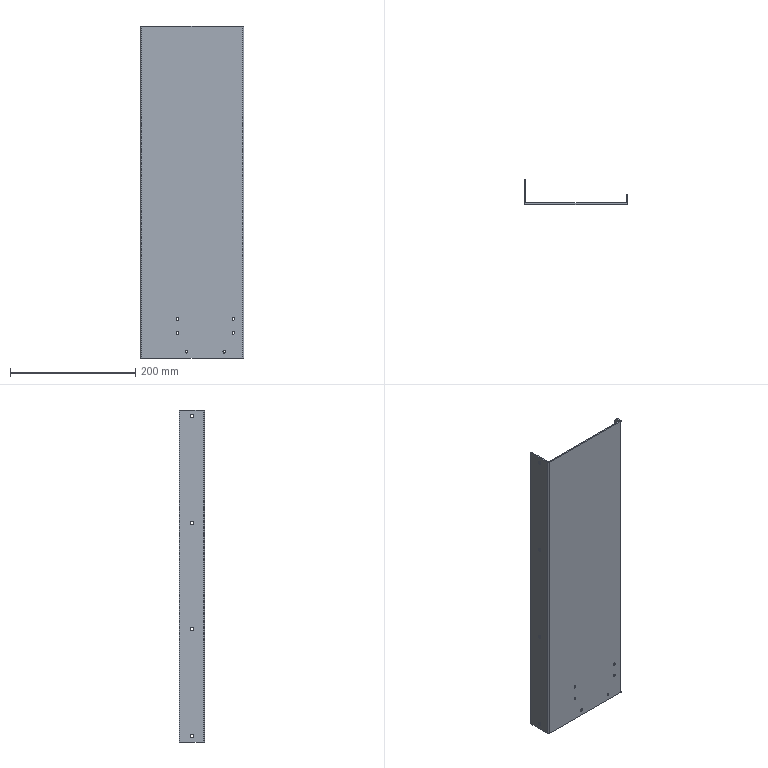Part | STEP file | 0245_217_Cable | 1 solid | 34 faces | box 165 x 40 x 530 mm | volume 227644 mm3 | cylinder 22 | plane 12 | commonest cylinder face diameters 4.2 x12 5.5 x8 4 x2